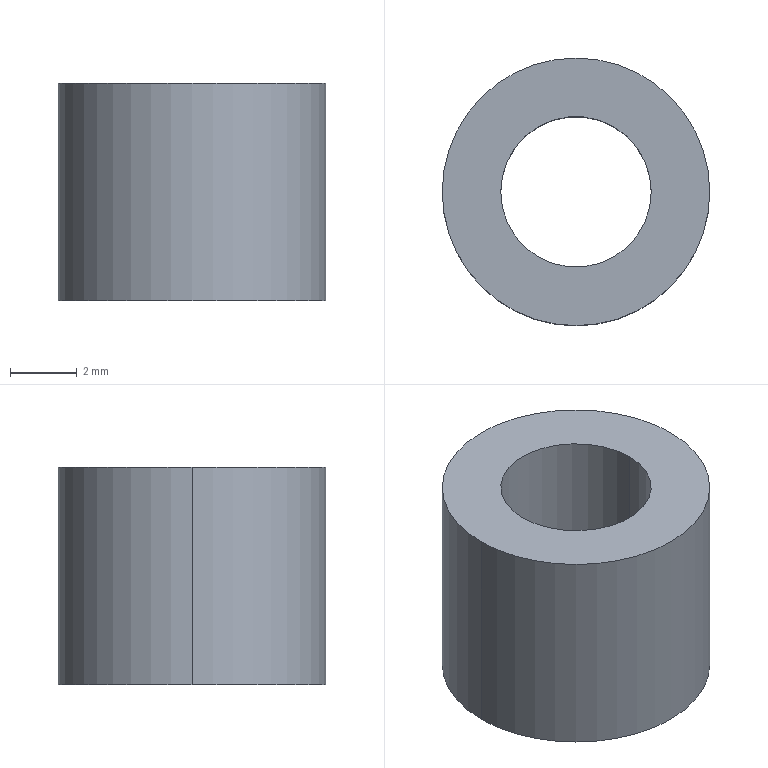Part | SolidWorks | features Extrusion 1, ICE 1 | 1 solid | 6 faces | box 8 x 8 x 6.5 mm | volume 223.348 mm3 | cylinder 4 | plane 2 | commonest cylinder face diameters 4.5 x2 8 x2
STEP:
#1=CARTESIAN_POINT('',(-2.25,0.,0.));
#2=VERTEX_POINT('',#1);
#3=CARTESIAN_POINT('',(2.25,0.,0.));
#4=VERTEX_POINT('',#3);
#5=CARTESIAN_POINT('',(0.,0.,0.));
#6=DIRECTION('',(0.,0.,1.));
#7=DIRECTION('',(1.,0.,0.));
#8=AXIS2_PLACEMENT_3D('',#5,#6,#7);
#9=CIRCLE('',#8,2.25);
#10=EDGE_CURVE('',#2,#4,#9,.T.);
#11=ORIENTED_EDGE('',*,*,#10,.F.);
#12=CARTESIAN_POINT('',(-2.25,0.,6.5));
#13=VERTEX_POINT('',#12);
#14=CARTESIAN_POINT('',(-2.25,0.,0.));
#15=DIRECTION('',(0.,0.,1.));
#16=VECTOR('',#15,1000.);
#17=LINE('',#14,#16);
#18=EDGE_CURVE('',#2,#13,#17,.T.);
#19=ORIENTED_EDGE('',*,*,#18,.T.);
#20=CARTESIAN_POINT('',(2.25,0.,6.5));
#21=VERTEX_POINT('',#20);
#22=CARTESIAN_POINT('',(0.,0.,6.5));
#23=DIRECTION('',(0.,0.,1.));
#24=DIRECTION('',(1.,0.,0.));
#25=AXIS2_PLACEMENT_3D('',#22,#23,#24);
#26=CIRCLE('',#25,2.25);
#27=EDGE_CURVE('',#13,#21,#26,.T.);
#28=ORIENTED_EDGE('',*,*,#27,.T.);
#29=CARTESIAN_POINT('',(2.25,0.,0.));
#30=DIRECTION('',(0.,0.,1.));
#31=VECTOR('',#30,1000.);
#32=LINE('',#29,#31);
#33=EDGE_CURVE('',#4,#21,#32,.T.);
#34=ORIENTED_EDGE('',*,*,#33,.F.);
#35=EDGE_LOOP('',(#11,#19,#28,#34));
#36=FACE_OUTER_BOUND('',#35,.T.);
#37=CARTESIAN_POINT('',(0.,0.,0.));
#38=DIRECTION('',(0.,0.,1.));
#39=DIRECTION('',(1.,0.,0.));
#40=AXIS2_PLACEMENT_3D('',#37,#38,#39);
#41=CYLINDRICAL_SURFACE('',#40,2.25);
#42=ADVANCED_FACE('',(#36),#41,.F.);
#43=CARTESIAN_POINT('',(4.,0.,6.5));
#44=VERTEX_POINT('',#43);
#45=CARTESIAN_POINT('',(-4.,0.,6.5));
#46=VERTEX_POINT('',#45);
#47=CARTESIAN_POINT('',(0.,0.,6.5));
#48=DIRECTION('',(0.,0.,1.));
#49=DIRECTION('',(1.,0.,0.));
#50=AXIS2_PLACEMENT_3D('',#47,#48,#49);
#51=CIRCLE('',#50,4.);
#52=EDGE_CURVE('',#44,#46,#51,.T.);
#53=ORIENTED_EDGE('',*,*,#52,.F.);
#54=CARTESIAN_POINT('',(4.,0.,0.));
#55=VERTEX_POINT('',#54);
#56=CARTESIAN_POINT('',(4.,0.,6.5));
#57=DIRECTION('',(0.,0.,-1.));
#58=VECTOR('',#57,1000.);
#59=LINE('',#56,#58);
#60=EDGE_CURVE('',#44,#55,#59,.T.);
#61=ORIENTED_EDGE('',*,*,#60,.T.);
#62=CARTESIAN_POINT('',(-4.,0.,0.));
#63=VERTEX_POINT('',#62);
#64=CARTESIAN_POINT('',(0.,0.,0.));
#65=DIRECTION('',(0.,0.,1.));
#66=DIRECTION('',(1.,0.,0.));
#67=AXIS2_PLACEMENT_3D('',#64,#65,#66);
#68=CIRCLE('',#67,4.);
#69=EDGE_CURVE('',#55,#63,#68,.T.);
#70=ORIENTED_EDGE('',*,*,#69,.T.);
#71=CARTESIAN_POINT('',(-4.,0.,6.5));
#72=DIRECTION('',(0.,0.,-1.));
#73=VECTOR('',#72,1000.);
#74=LINE('',#71,#73);
#75=EDGE_CURVE('',#46,#63,#74,.T.);
#76=ORIENTED_EDGE('',*,*,#75,.F.);
#77=EDGE_LOOP('',(#53,#61,#70,#76));
#78=FACE_OUTER_BOUND('',#77,.T.);
#79=CARTESIAN_POINT('',(0.,0.,6.5));
#80=DIRECTION('',(0.,0.,-1.));
#81=DIRECTION('',(-1.,0.,0.));
#82=AXIS2_PLACEMENT_3D('',#79,#80,#81);
#83=CYLINDRICAL_SURFACE('',#82,4.);
#84=ADVANCED_FACE('',(#78),#83,.T.);
#85=ORIENTED_EDGE('',*,*,#60,.F.);
#86=CARTESIAN_POINT('',(0.,0.,6.5));
#87=DIRECTION('',(0.,0.,1.));
#88=DIRECTION('',(1.,0.,0.));
#89=AXIS2_PLACEMENT_3D('',#86,#87,#88);
#90=CIRCLE('',#89,4.);
#91=EDGE_CURVE('',#46,#44,#90,.T.);
#92=ORIENTED_EDGE('',*,*,#91,.F.);
#93=ORIENTED_EDGE('',*,*,#75,.T.);
#94=CARTESIAN_POINT('',(0.,0.,0.));
#95=DIRECTION('',(0.,0.,1.));
#96=DIRECTION('',(1.,0.,0.));
#97=AXIS2_PLACEMENT_3D('',#94,#95,#96);
#98=CIRCLE('',#97,4.);
#99=EDGE_CURVE('',#63,#55,#98,.T.);
#100=ORIENTED_EDGE('',*,*,#99,.T.);
#101=EDGE_LOOP('',(#85,#92,#93,#100));
#102=FACE_OUTER_BOUND('',#101,.T.);
#103=CARTESIAN_POINT('',(0.,0.,6.5));
#104=DIRECTION('',(0.,0.,-1.));
#105=DIRECTION('',(-1.,0.,0.));
#106=AXIS2_PLACEMENT_3D('',#103,#104,#105);
#107=CYLINDRICAL_SURFACE('',#106,4.);
#108=ADVANCED_FACE('',(#102),#107,.T.);
#109=CARTESIAN_POINT('',(0.,0.,6.5));
#110=DIRECTION('',(0.,0.,1.));
#111=DIRECTION('',(1.,0.,0.));
#112=AXIS2_PLACEMENT_3D('',#109,#110,#111);
#113=CIRCLE('',#112,2.25);
#114=EDGE_CURVE('',#21,#13,#113,.T.);
#115=ORIENTED_EDGE('',*,*,#114,.F.);
#116=ORIENTED_EDGE('',*,*,#27,.F.);
#117=EDGE_LOOP('',(#115,#116));
#118=FACE_BOUND('',#117,.T.);
#119=ORIENTED_EDGE('',*,*,#91,.T.);
#120=ORIENTED_EDGE('',*,*,#52,.T.);
#121=EDGE_LOOP('',(#119,#120));
#122=FACE_OUTER_BOUND('',#121,.T.);
#123=CARTESIAN_POINT('',(0.,0.,6.5));
#124=DIRECTION('',(0.,0.,1.));
#125=DIRECTION('',(1.,0.,0.));
#126=AXIS2_PLACEMENT_3D('',#123,#124,#125);
#127=PLANE('',#126);
#128=ADVANCED_FACE('',(#118,#122),#127,.T.);
#129=CARTESIAN_POINT('',(0.,0.,0.));
#130=DIRECTION('',(0.,0.,1.));
#131=DIRECTION('',(1.,0.,0.));
#132=AXIS2_PLACEMENT_3D('',#129,#130,#131);
#133=CIRCLE('',#132,2.25);
#134=EDGE_CURVE('',#4,#2,#133,.T.);
#135=ORIENTED_EDGE('',*,*,#134,.T.);
#136=ORIENTED_EDGE('',*,*,#10,.T.);
#137=EDGE_LOOP('',(#135,#136));
#138=FACE_BOUND('',#137,.T.);
#139=ORIENTED_EDGE('',*,*,#99,.F.);
#140=ORIENTED_EDGE('',*,*,#69,.F.);
#141=EDGE_LOOP('',(#139,#140));
#142=FACE_OUTER_BOUND('',#141,.T.);
#143=CARTESIAN_POINT('',(0.,0.,0.));
#144=DIRECTION('',(0.,0.,1.));
#145=DIRECTION('',(1.,0.,0.));
#146=AXIS2_PLACEMENT_3D('',#143,#144,#145);
#147=PLANE('',#146);
#148=ADVANCED_FACE('',(#138,#142),#147,.F.);
#149=ORIENTED_EDGE('',*,*,#18,.F.);
#150=ORIENTED_EDGE('',*,*,#134,.F.);
#151=ORIENTED_EDGE('',*,*,#33,.T.);
#152=ORIENTED_EDGE('',*,*,#114,.T.);
#153=EDGE_LOOP('',(#149,#150,#151,#152));
#154=FACE_OUTER_BOUND('',#153,.T.);
#155=CARTESIAN_POINT('',(0.,0.,0.));
#156=DIRECTION('',(0.,0.,1.));
#157=DIRECTION('',(1.,0.,0.));
#158=AXIS2_PLACEMENT_3D('',#155,#156,#157);
#159=CYLINDRICAL_SURFACE('',#158,2.25);
#160=ADVANCED_FACE('',(#154),#159,.F.);
#161=CLOSED_SHELL('',(#42,#84,#108,#128,#148,#160));
#162=MANIFOLD_SOLID_BREP('',#161);
#163=CARTESIAN_POINT('',(0.,0.,0.));
#164=DIRECTION('',(0.,0.,1.));
#165=DIRECTION('',(1.,0.,0.));
#166=AXIS2_PLACEMENT_3D('',#163,#164,#165);
#167=(LENGTH_UNIT()NAMED_UNIT(*)SI_UNIT(.MILLI.,.METRE.));
#168=UNCERTAINTY_MEASURE_WITH_UNIT(LENGTH_MEASURE(0.00001),#167,'','');
#169=(NAMED_UNIT(*)PLANE_ANGLE_UNIT()SI_UNIT($,.RADIAN.));
#170=(NAMED_UNIT(*)SI_UNIT($,.STERADIAN.)SOLID_ANGLE_UNIT());
#171=(GEOMETRIC_REPRESENTATION_CONTEXT(3)GLOBAL_UNCERTAINTY_ASSIGNED_CONTEXT((#168))GLOBAL_UNIT_ASSIGNED_CONTEXT((#167,#169,#170))REPRESENTATION_CONTEXT('',''));
#172=ADVANCED_BREP_SHAPE_REPRESENTATION('',(#162,#166),#171);